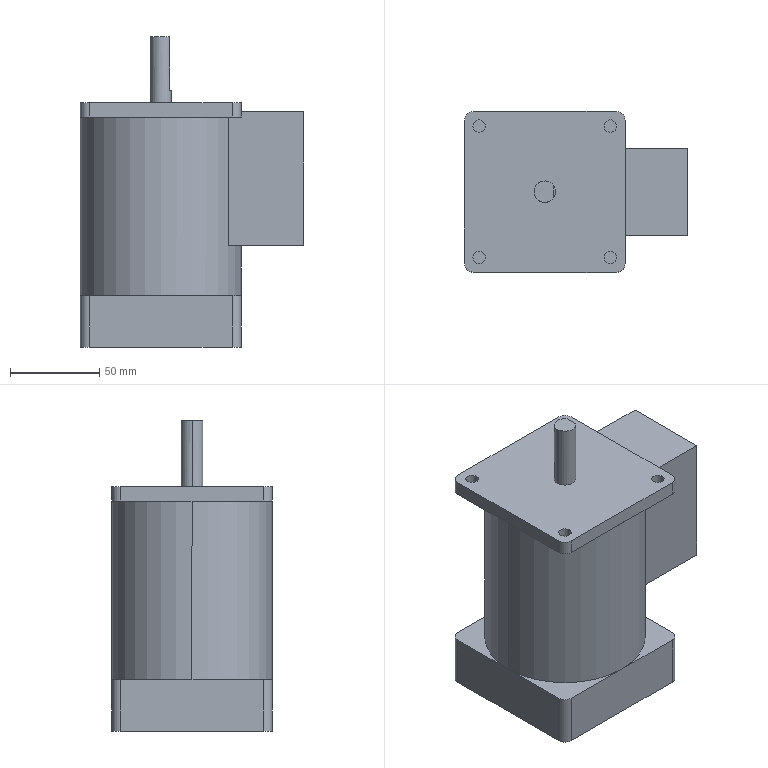Part | SolidWorks | features ICE 6, Fillet 2, CirPattern 1, Extrusion 1 | 1 solid | 46 faces | box 125 x 90 x 174 mm | volume 1074757 mm3 | plane 26 | cylinder 20 | commonest cylinder face diameters 7 x8 10 x8 12 x2 90 x2
STEP:
#1=CARTESIAN_POINT('',(40.27,36.77,0.));
#2=VERTEX_POINT('',#1);
#3=CARTESIAN_POINT('',(33.27,36.77,0.));
#4=VERTEX_POINT('',#3);
#5=CARTESIAN_POINT('',(36.77,36.77,0.));
#6=DIRECTION('',(0.,0.,-1.));
#7=DIRECTION('',(1.,0.,0.));
#8=AXIS2_PLACEMENT_3D('',#5,#6,#7);
#9=CIRCLE('',#8,3.5);
#10=EDGE_CURVE('',#2,#4,#9,.T.);
#11=ORIENTED_EDGE('',*,*,#10,.T.);
#12=CARTESIAN_POINT('',(33.27,36.77,8.));
#13=VERTEX_POINT('',#12);
#14=CARTESIAN_POINT('',(33.27,36.77,-9.899));
#15=DIRECTION('',(0.,0.,1.));
#16=VECTOR('',#15,1000.);
#17=LINE('',#14,#16);
#18=EDGE_CURVE('',#4,#13,#17,.T.);
#19=ORIENTED_EDGE('',*,*,#18,.T.);
#20=CARTESIAN_POINT('',(40.27,36.77,8.));
#21=VERTEX_POINT('',#20);
#22=CARTESIAN_POINT('',(36.77,36.77,8.));
#23=DIRECTION('',(0.,0.,1.));
#24=DIRECTION('',(0.,-1.,0.));
#25=AXIS2_PLACEMENT_3D('',#22,#23,#24);
#26=CIRCLE('',#25,3.5);
#27=EDGE_CURVE('',#13,#21,#26,.T.);
#28=ORIENTED_EDGE('',*,*,#27,.T.);
#29=CARTESIAN_POINT('',(40.27,36.77,-9.899));
#30=DIRECTION('',(0.,0.,1.));
#31=VECTOR('',#30,1000.);
#32=LINE('',#29,#31);
#33=EDGE_CURVE('',#2,#21,#32,.T.);
#34=ORIENTED_EDGE('',*,*,#33,.F.);
#35=EDGE_LOOP('',(#11,#19,#28,#34));
#36=FACE_OUTER_BOUND('',#35,.T.);
#37=CARTESIAN_POINT('',(36.77,36.77,-9.899));
#38=DIRECTION('',(0.,0.,1.));
#39=DIRECTION('',(1.,0.,0.));
#40=AXIS2_PLACEMENT_3D('',#37,#38,#39);
#41=CYLINDRICAL_SURFACE('',#40,3.5);
#42=ADVANCED_FACE('',(#36),#41,.F.);
#43=CARTESIAN_POINT('',(40.27,-36.77,0.));
#44=VERTEX_POINT('',#43);
#45=CARTESIAN_POINT('',(33.27,-36.77,0.));
#46=VERTEX_POINT('',#45);
#47=CARTESIAN_POINT('',(36.77,-36.77,0.));
#48=DIRECTION('',(0.,0.,-1.));
#49=DIRECTION('',(1.,0.,0.));
#50=AXIS2_PLACEMENT_3D('',#47,#48,#49);
#51=CIRCLE('',#50,3.5);
#52=EDGE_CURVE('',#44,#46,#51,.T.);
#53=ORIENTED_EDGE('',*,*,#52,.T.);
#54=CARTESIAN_POINT('',(33.27,-36.77,8.));
#55=VERTEX_POINT('',#54);
#56=CARTESIAN_POINT('',(33.27,-36.77,-9.899));
#57=DIRECTION('',(0.,0.,1.));
#58=VECTOR('',#57,1000.);
#59=LINE('',#56,#58);
#60=EDGE_CURVE('',#46,#55,#59,.T.);
#61=ORIENTED_EDGE('',*,*,#60,.T.);
#62=CARTESIAN_POINT('',(40.27,-36.77,8.));
#63=VERTEX_POINT('',#62);
#64=CARTESIAN_POINT('',(36.77,-36.77,8.));
#65=DIRECTION('',(0.,0.,1.));
#66=DIRECTION('',(-1.,0.,0.));
#67=AXIS2_PLACEMENT_3D('',#64,#65,#66);
#68=CIRCLE('',#67,3.5);
#69=EDGE_CURVE('',#55,#63,#68,.T.);
#70=ORIENTED_EDGE('',*,*,#69,.T.);
#71=CARTESIAN_POINT('',(40.27,-36.77,-9.899));
#72=DIRECTION('',(0.,0.,1.));
#73=VECTOR('',#72,1000.);
#74=LINE('',#71,#73);
#75=EDGE_CURVE('',#44,#63,#74,.T.);
#76=ORIENTED_EDGE('',*,*,#75,.F.);
#77=EDGE_LOOP('',(#53,#61,#70,#76));
#78=FACE_OUTER_BOUND('',#77,.T.);
#79=CARTESIAN_POINT('',(36.77,-36.77,-9.899));
#80=DIRECTION('',(0.,0.,1.));
#81=DIRECTION('',(1.,0.,0.));
#82=AXIS2_PLACEMENT_3D('',#79,#80,#81);
#83=CYLINDRICAL_SURFACE('',#82,3.5);
#84=ADVANCED_FACE('',(#78),#83,.F.);
#85=CARTESIAN_POINT('',(-33.27,-36.77,0.));
#86=VERTEX_POINT('',#85);
#87=CARTESIAN_POINT('',(-40.27,-36.77,0.));
#88=VERTEX_POINT('',#87);
#89=CARTESIAN_POINT('',(-36.77,-36.77,0.));
#90=DIRECTION('',(0.,0.,-1.));
#91=DIRECTION('',(1.,0.,0.));
#92=AXIS2_PLACEMENT_3D('',#89,#90,#91);
#93=CIRCLE('',#92,3.5);
#94=EDGE_CURVE('',#86,#88,#93,.T.);
#95=ORIENTED_EDGE('',*,*,#94,.T.);
#96=CARTESIAN_POINT('',(-40.27,-36.77,8.));
#97=VERTEX_POINT('',#96);
#98=CARTESIAN_POINT('',(-40.27,-36.77,-9.899));
#99=DIRECTION('',(0.,0.,1.));
#100=VECTOR('',#99,1000.);
#101=LINE('',#98,#100);
#102=EDGE_CURVE('',#88,#97,#101,.T.);
#103=ORIENTED_EDGE('',*,*,#102,.T.);
#104=CARTESIAN_POINT('',(-33.27,-36.77,8.));
#105=VERTEX_POINT('',#104);
#106=CARTESIAN_POINT('',(-36.77,-36.77,8.));
#107=DIRECTION('',(0.,0.,1.));
#108=DIRECTION('',(0.,1.,0.));
#109=AXIS2_PLACEMENT_3D('',#106,#107,#108);
#110=CIRCLE('',#109,3.5);
#111=EDGE_CURVE('',#97,#105,#110,.T.);
#112=ORIENTED_EDGE('',*,*,#111,.T.);
#113=CARTESIAN_POINT('',(-33.27,-36.77,-9.899));
#114=DIRECTION('',(0.,0.,1.));
#115=VECTOR('',#114,1000.);
#116=LINE('',#113,#115);
#117=EDGE_CURVE('',#86,#105,#116,.T.);
#118=ORIENTED_EDGE('',*,*,#117,.F.);
#119=EDGE_LOOP('',(#95,#103,#112,#118));
#120=FACE_OUTER_BOUND('',#119,.T.);
#121=CARTESIAN_POINT('',(-36.77,-36.77,-9.899));
#122=DIRECTION('',(0.,0.,1.));
#123=DIRECTION('',(1.,0.,0.));
#124=AXIS2_PLACEMENT_3D('',#121,#122,#123);
#125=CYLINDRICAL_SURFACE('',#124,3.5);
#126=ADVANCED_FACE('',(#120),#125,.F.);
#127=CARTESIAN_POINT('',(-33.27,36.77,0.));
#128=VERTEX_POINT('',#127);
#129=CARTESIAN_POINT('',(-40.27,36.77,0.));
#130=VERTEX_POINT('',#129);
#131=CARTESIAN_POINT('',(-36.77,36.77,0.));
#132=DIRECTION('',(0.,0.,-1.));
#133=DIRECTION('',(1.,0.,0.));
#134=AXIS2_PLACEMENT_3D('',#131,#132,#133);
#135=CIRCLE('',#134,3.5);
#136=EDGE_CURVE('',#128,#130,#135,.T.);
#137=ORIENTED_EDGE('',*,*,#136,.T.);
#138=CARTESIAN_POINT('',(-40.27,36.77,8.));
#139=VERTEX_POINT('',#138);
#140=CARTESIAN_POINT('',(-40.27,36.77,-9.899));
#141=DIRECTION('',(0.,0.,1.));
#142=VECTOR('',#141,1000.);
#143=LINE('',#140,#142);
#144=EDGE_CURVE('',#130,#139,#143,.T.);
#145=ORIENTED_EDGE('',*,*,#144,.T.);
#146=CARTESIAN_POINT('',(-33.27,36.77,8.));
#147=VERTEX_POINT('',#146);
#148=CARTESIAN_POINT('',(-36.77,36.77,8.));
#149=DIRECTION('',(0.,0.,1.));
#150=DIRECTION('',(1.,0.,0.));
#151=AXIS2_PLACEMENT_3D('',#148,#149,#150);
#152=CIRCLE('',#151,3.5);
#153=EDGE_CURVE('',#139,#147,#152,.T.);
#154=ORIENTED_EDGE('',*,*,#153,.T.);
#155=CARTESIAN_POINT('',(-33.27,36.77,-9.899));
#156=DIRECTION('',(0.,0.,1.));
#157=VECTOR('',#156,1000.);
#158=LINE('',#155,#157);
#159=EDGE_CURVE('',#128,#147,#158,.T.);
#160=ORIENTED_EDGE('',*,*,#159,.F.);
#161=EDGE_LOOP('',(#137,#145,#154,#160));
#162=FACE_OUTER_BOUND('',#161,.T.);
#163=CARTESIAN_POINT('',(-36.77,36.77,-9.899));
#164=DIRECTION('',(0.,0.,1.));
#165=DIRECTION('',(1.,0.,0.));
#166=AXIS2_PLACEMENT_3D('',#163,#164,#165);
#167=CYLINDRICAL_SURFACE('',#166,3.5);
#168=ADVANCED_FACE('',(#162),#167,.F.);
#169=CARTESIAN_POINT('',(-45.,0.,-100.));
#170=VERTEX_POINT('',#169);
#171=CARTESIAN_POINT('',(0.,45.,-100.));
#172=VERTEX_POINT('',#171);
#173=CARTESIAN_POINT('',(0.,0.,-100.));
#174=DIRECTION('',(0.,0.,-1.));
#175=DIRECTION('',(-1.,0.,0.));
#176=AXIS2_PLACEMENT_3D('',#173,#174,#175);
#177=CIRCLE('',#176,45.);
#178=EDGE_CURVE('',#170,#172,#177,.T.);
#179=ORIENTED_EDGE('',*,*,#178,.F.);
#180=CARTESIAN_POINT('',(-45.,0.,0.));
#181=VERTEX_POINT('',#180);
#182=CARTESIAN_POINT('',(-45.,0.,-100.));
#183=DIRECTION('',(0.,0.,1.));
#184=VECTOR('',#183,1000.);
#185=LINE('',#182,#184);
#186=EDGE_CURVE('',#170,#181,#185,.T.);
#187=ORIENTED_EDGE('',*,*,#186,.T.);
#188=CARTESIAN_POINT('',(0.,45.,0.));
#189=VERTEX_POINT('',#188);
#190=CARTESIAN_POINT('',(0.,0.,0.));
#191=DIRECTION('',(0.,0.,-1.));
#192=DIRECTION('',(-1.,0.,0.));
#193=AXIS2_PLACEMENT_3D('',#190,#191,#192);
#194=CIRCLE('',#193,45.);
#195=EDGE_CURVE('',#181,#189,#194,.T.);
#196=ORIENTED_EDGE('',*,*,#195,.T.);
#197=CARTESIAN_POINT('',(37.746,24.5,0.));
#198=VERTEX_POINT('',#197);
#199=CARTESIAN_POINT('',(0.,0.,0.));
#200=DIRECTION('',(0.,0.,-1.));
#201=DIRECTION('',(-1.,0.,0.));
#202=AXIS2_PLACEMENT_3D('',#199,#200,#201);
#203=CIRCLE('',#202,45.);
#204=EDGE_CURVE('',#189,#198,#203,.T.);
#205=ORIENTED_EDGE('',*,*,#204,.T.);
#206=CARTESIAN_POINT('',(37.746,24.5,-72.));
#207=VERTEX_POINT('',#206);
#208=CARTESIAN_POINT('',(37.746,24.5,-100.));
#209=DIRECTION('',(0.,0.,1.));
#210=VECTOR('',#209,1000.);
#211=LINE('',#208,#210);
#212=EDGE_CURVE('',#207,#198,#211,.T.);
#213=ORIENTED_EDGE('',*,*,#212,.F.);
#214=CARTESIAN_POINT('',(45.,0.,-72.));
#215=VERTEX_POINT('',#214);
#216=CARTESIAN_POINT('',(0.,0.,-72.));
#217=DIRECTION('',(0.,0.,1.));
#218=DIRECTION('',(1.,0.,0.));
#219=AXIS2_PLACEMENT_3D('',#216,#217,#218);
#220=CIRCLE('',#219,45.);
#221=EDGE_CURVE('',#215,#207,#220,.T.);
#222=ORIENTED_EDGE('',*,*,#221,.F.);
#223=CARTESIAN_POINT('',(45.,0.,-100.));
#224=VERTEX_POINT('',#223);
#225=CARTESIAN_POINT('',(45.,0.,-100.));
#226=DIRECTION('',(0.,0.,1.));
#227=VECTOR('',#226,1000.);
#228=LINE('',#225,#227);
#229=EDGE_CURVE('',#224,#215,#228,.T.);
#230=ORIENTED_EDGE('',*,*,#229,.F.);
#231=CARTESIAN_POINT('',(0.,0.,-100.));
#232=DIRECTION('',(0.,0.,-1.));
#233=DIRECTION('',(-1.,0.,0.));
#234=AXIS2_PLACEMENT_3D('',#231,#232,#233);
#235=CIRCLE('',#234,45.);
#236=EDGE_CURVE('',#172,#224,#235,.T.);
#237=ORIENTED_EDGE('',*,*,#236,.F.);
#238=EDGE_LOOP('',(#179,#187,#196,#205,#213,#222,#230,#237));
#239=FACE_OUTER_BOUND('',#238,.T.);
#240=CARTESIAN_POINT('',(0.,0.,-100.));
#241=DIRECTION('',(0.,0.,1.));
#242=DIRECTION('',(1.,0.,0.));
#243=AXIS2_PLACEMENT_3D('',#240,#241,#242);
#244=CYLINDRICAL_SURFACE('',#243,45.);
#245=ADVANCED_FACE('',(#239),#244,.T.);
#246=CARTESIAN_POINT('',(5.,3.317,15.));
#247=VERTEX_POINT('',#246);
#248=CARTESIAN_POINT('',(6.,0.,15.));
#249=VERTEX_POINT('',#248);
#250=CARTESIAN_POINT('',(0.,0.,15.));
#251=DIRECTION('',(0.,0.,-1.));
#252=DIRECTION('',(0.,1.,0.));
#253=AXIS2_PLACEMENT_3D('',#250,#251,#252);
#254=CIRCLE('',#253,6.);
#255=EDGE_CURVE('',#247,#249,#254,.T.);
#256=ORIENTED_EDGE('',*,*,#255,.T.);
#257=CARTESIAN_POINT('',(6.,0.,8.));
#258=VERTEX_POINT('',#257);
#259=CARTESIAN_POINT('',(6.,0.,45.));
#260=DIRECTION('',(0.,0.,-1.));
#261=VECTOR('',#260,1000.);
#262=LINE('',#259,#261);
#263=EDGE_CURVE('',#249,#258,#262,.T.);
#264=ORIENTED_EDGE('',*,*,#263,.T.);
#265=CARTESIAN_POINT('',(-6.,0.,8.));
#266=VERTEX_POINT('',#265);
#267=CARTESIAN_POINT('',(0.,0.,8.));
#268=DIRECTION('',(0.,0.,1.));
#269=DIRECTION('',(1.,0.,0.));
#270=AXIS2_PLACEMENT_3D('',#267,#268,#269);
#271=CIRCLE('',#270,6.);
#272=EDGE_CURVE('',#258,#266,#271,.T.);
#273=ORIENTED_EDGE('',*,*,#272,.T.);
#274=CARTESIAN_POINT('',(-6.,0.,45.));
#275=VERTEX_POINT('',#274);
#276=CARTESIAN_POINT('',(-6.,0.,45.));
#277=DIRECTION('',(0.,0.,-1.));
#278=VECTOR('',#277,1000.);
#279=LINE('',#276,#278);
#280=EDGE_CURVE('',#275,#266,#279,.T.);
#281=ORIENTED_EDGE('',*,*,#280,.F.);
#282=CARTESIAN_POINT('',(5.,3.317,45.));
#283=VERTEX_POINT('',#282);
#284=CARTESIAN_POINT('',(0.,0.,45.));
#285=DIRECTION('',(0.,0.,1.));
#286=DIRECTION('',(1.,0.,0.));
#287=AXIS2_PLACEMENT_3D('',#284,#285,#286);
#288=CIRCLE('',#287,6.);
#289=EDGE_CURVE('',#283,#275,#288,.T.);
#290=ORIENTED_EDGE('',*,*,#289,.F.);
#291=CARTESIAN_POINT('',(5.,3.317,45.));
#292=DIRECTION('',(0.,0.,1.));
#293=VECTOR('',#292,1000.);
#294=LINE('',#291,#293);
#295=EDGE_CURVE('',#247,#283,#294,.T.);
#296=ORIENTED_EDGE('',*,*,#295,.F.);
#297=EDGE_LOOP('',(#256,#264,#273,#281,#290,#296));
#298=FACE_OUTER_BOUND('',#297,.T.);
#299=CARTESIAN_POINT('',(0.,0.,45.));
#300=DIRECTION('',(0.,0.,-1.));
#301=DIRECTION('',(-1.,0.,0.));
#302=AXIS2_PLACEMENT_3D('',#299,#300,#301);
#303=CYLINDRICAL_SURFACE('',#302,6.);
#304=ADVANCED_FACE('',(#298),#303,.T.);
#305=ORIENTED_EDGE('',*,*,#263,.F.);
#306=CARTESIAN_POINT('',(5.,-3.317,15.));
#307=VERTEX_POINT('',#306);
#308=CARTESIAN_POINT('',(0.,0.,15.));
#309=DIRECTION('',(0.,0.,-1.));
#310=DIRECTION('',(0.,1.,0.));
#311=AXIS2_PLACEMENT_3D('',#308,#309,#310);
#312=CIRCLE('',#311,6.);
#313=EDGE_CURVE('',#249,#307,#312,.T.);
#314=ORIENTED_EDGE('',*,*,#313,.T.);
#315=CARTESIAN_POINT('',(5.,-3.317,45.));
#316=VERTEX_POINT('',#315);
#317=CARTESIAN_POINT('',(5.,-3.317,45.));
#318=DIRECTION('',(0.,0.,-1.));
#319=VECTOR('',#318,1000.);
#320=LINE('',#317,#319);
#321=EDGE_CURVE('',#316,#307,#320,.T.);
#322=ORIENTED_EDGE('',*,*,#321,.F.);
#323=CARTESIAN_POINT('',(0.,0.,45.));
#324=DIRECTION('',(0.,0.,1.));
#325=DIRECTION('',(1.,0.,0.));
#326=AXIS2_PLACEMENT_3D('',#323,#324,#325);
#327=CIRCLE('',#326,6.);
#328=EDGE_CURVE('',#275,#316,#327,.T.);
#329=ORIENTED_EDGE('',*,*,#328,.F.);
#330=ORIENTED_EDGE('',*,*,#280,.T.);
#331=CARTESIAN_POINT('',(0.,0.,8.));
#332=DIRECTION('',(0.,0.,1.));
#333=DIRECTION('',(1.,0.,0.));
#334=AXIS2_PLACEMENT_3D('',#331,#332,#333);
#335=CIRCLE('',#334,6.);
#336=EDGE_CURVE('',#266,#258,#335,.T.);
#337=ORIENTED_EDGE('',*,*,#336,.T.);
#338=EDGE_LOOP('',(#305,#314,#322,#329,#330,#337));
#339=FACE_OUTER_BOUND('',#338,.T.);
#340=CARTESIAN_POINT('',(0.,0.,45.));
#341=DIRECTION('',(0.,0.,-1.));
#342=DIRECTION('',(-1.,0.,0.));
#343=AXIS2_PLACEMENT_3D('',#340,#341,#342);
#344=CYLINDRICAL_SURFACE('',#343,6.);
#345=ADVANCED_FACE('',(#339),#344,.T.);
#346=ORIENTED_EDGE('',*,*,#289,.T.);
#347=ORIENTED_EDGE('',*,*,#328,.T.);
#348=CARTESIAN_POINT('',(5.,0.,45.));
#349=DIRECTION('',(0.,1.,0.));
#350=VECTOR('',#349,1000.);
#351=LINE('',#348,#350);
#352=EDGE_CURVE('',#316,#283,#351,.T.);
#353=ORIENTED_EDGE('',*,*,#352,.T.);
#354=EDGE_LOOP('',(#346,#347,#353));
#355=FACE_OUTER_BOUND('',#354,.T.);
#356=CARTESIAN_POINT('',(0.,0.,45.));
#357=DIRECTION('',(0.,0.,1.));
#358=DIRECTION('',(1.,0.,0.));
#359=AXIS2_PLACEMENT_3D('',#356,#357,#358);
#360=PLANE('',#359);
#361=ADVANCED_FACE('',(#355),#360,.T.);
#362=ORIENTED_EDGE('',*,*,#10,.F.);
#363=CARTESIAN_POINT('',(36.77,36.77,0.));
#364=DIRECTION('',(0.,0.,-1.));
#365=DIRECTION('',(1.,0.,0.));
#366=AXIS2_PLACEMENT_3D('',#363,#364,#365);
#367=CIRCLE('',#366,3.5);
#368=EDGE_CURVE('',#4,#2,#367,.T.);
#369=ORIENTED_EDGE('',*,*,#368,.F.);
#370=EDGE_LOOP('',(#362,#369));
#371=FACE_BOUND('',#370,.T.);
#372=CARTESIAN_POINT('',(40.,45.,0.));
#373=VERTEX_POINT('',#372);
#374=CARTESIAN_POINT('',(-45.,45.,0.));
#375=DIRECTION('',(-1.,0.,0.));
#376=VECTOR('',#375,1000.);
#377=LINE('',#374,#376);
#378=EDGE_CURVE('',#373,#189,#377,.T.);
#379=ORIENTED_EDGE('',*,*,#378,.F.);
#380=CARTESIAN_POINT('',(45.,40.,0.));
#381=VERTEX_POINT('',#380);
#382=CARTESIAN_POINT('',(40.,40.,0.));
#383=DIRECTION('',(0.,0.,-1.));
#384=DIRECTION('',(1.,0.,0.));
#385=AXIS2_PLACEMENT_3D('',#382,#383,#384);
#386=CIRCLE('',#385,5.);
#387=EDGE_CURVE('',#373,#381,#386,.T.);
#388=ORIENTED_EDGE('',*,*,#387,.T.);
#389=CARTESIAN_POINT('',(45.,24.5,0.));
#390=VERTEX_POINT('',#389);
#391=CARTESIAN_POINT('',(45.,45.,0.));
#392=DIRECTION('',(0.,1.,0.));
#393=VECTOR('',#392,1000.);
#394=LINE('',#391,#393);
#395=EDGE_CURVE('',#390,#381,#394,.T.);
#396=ORIENTED_EDGE('',*,*,#395,.F.);
#397=CARTESIAN_POINT('',(-45.,24.5,0.));
#398=DIRECTION('',(1.,0.,0.));
#399=VECTOR('',#398,1000.);
#400=LINE('',#397,#399);
#401=EDGE_CURVE('',#198,#390,#400,.T.);
#402=ORIENTED_EDGE('',*,*,#401,.F.);
#403=ORIENTED_EDGE('',*,*,#204,.F.);
#404=EDGE_LOOP('',(#379,#388,#396,#402,#403));
#405=FACE_OUTER_BOUND('',#404,.T.);
#406=CARTESIAN_POINT('',(-45.,-45.,0.));
#407=DIRECTION('',(0.,0.,1.));
#408=DIRECTION('',(1.,0.,0.));
#409=AXIS2_PLACEMENT_3D('',#406,#407,#408);
#410=PLANE('',#409);
#411=ADVANCED_FACE('',(#371,#405),#410,.F.);
#412=ORIENTED_EDGE('',*,*,#52,.F.);
#413=CARTESIAN_POINT('',(36.77,-36.77,0.));
#414=DIRECTION('',(0.,0.,-1.));
#415=DIRECTION('',(1.,0.,0.));
#416=AXIS2_PLACEMENT_3D('',#413,#414,#415);
#417=CIRCLE('',#416,3.5);
#418=EDGE_CURVE('',#46,#44,#417,.T.);
#419=ORIENTED_EDGE('',*,*,#418,.F.);
#420=EDGE_LOOP('',(#412,#419));
#421=FACE_BOUND('',#420,.T.);
#422=CARTESIAN_POINT('',(45.,-40.,0.));
#423=VERTEX_POINT('',#422);
#424=CARTESIAN_POINT('',(45.,-24.5,0.));
#425=VERTEX_POINT('',#424);
#426=CARTESIAN_POINT('',(45.,45.,0.));
#427=DIRECTION('',(0.,1.,0.));
#428=VECTOR('',#427,1000.);
#429=LINE('',#426,#428);
#430=EDGE_CURVE('',#423,#425,#429,.T.);
#431=ORIENTED_EDGE('',*,*,#430,.F.);
#432=CARTESIAN_POINT('',(40.,-45.,0.));
#433=VERTEX_POINT('',#432);
#434=CARTESIAN_POINT('',(40.,-40.,0.));
#435=DIRECTION('',(0.,0.,-1.));
#436=DIRECTION('',(1.,0.,0.));
#437=AXIS2_PLACEMENT_3D('',#434,#435,#436);
#438=CIRCLE('',#437,5.);
#439=EDGE_CURVE('',#423,#433,#438,.T.);
#440=ORIENTED_EDGE('',*,*,#439,.T.);
#441=CARTESIAN_POINT('',(0.,-45.,0.));
#442=VERTEX_POINT('',#441);
#443=CARTESIAN_POINT('',(-45.,-45.,0.));
#444=DIRECTION('',(1.,0.,0.));
#445=VECTOR('',#444,1000.);
#446=LINE('',#443,#445);
#447=EDGE_CURVE('',#442,#433,#446,.T.);
#448=ORIENTED_EDGE('',*,*,#447,.F.);
#449=CARTESIAN_POINT('',(37.746,-24.5,0.));
#450=VERTEX_POINT('',#449);
#451=CARTESIAN_POINT('',(0.,0.,0.));
#452=DIRECTION('',(0.,0.,-1.));
#453=DIRECTION('',(-1.,0.,0.));
#454=AXIS2_PLACEMENT_3D('',#451,#452,#453);
#455=CIRCLE('',#454,45.);
#456=EDGE_CURVE('',#450,#442,#455,.T.);
#457=ORIENTED_EDGE('',*,*,#456,.F.);
#458=CARTESIAN_POINT('',(-45.,-24.5,0.));
#459=DIRECTION('',(-1.,0.,0.));
#460=VECTOR('',#459,1000.);
#461=LINE('',#458,#460);
#462=EDGE_CURVE('',#425,#450,#461,.T.);
#463=ORIENTED_EDGE('',*,*,#462,.F.);
#464=EDGE_LOOP('',(#431,#440,#448,#457,#463));
#465=FACE_OUTER_BOUND('',#464,.T.);
#466=CARTESIAN_POINT('',(-45.,-45.,0.));
#467=DIRECTION('',(0.,0.,1.));
#468=DIRECTION('',(1.,0.,0.));
#469=AXIS2_PLACEMENT_3D('',#466,#467,#468);
#470=PLANE('',#469);
#471=ADVANCED_FACE('',(#421,#465),#470,.F.);
#472=CARTESIAN_POINT('',(45.,-40.,8.));
#473=VERTEX_POINT('',#472);
#474=CARTESIAN_POINT('',(45.,40.,8.));
#475=VERTEX_POINT('',#474);
#476=CARTESIAN_POINT('',(45.,45.,8.));
#477=DIRECTION('',(0.,1.,0.));
#478=VECTOR('',#477,1000.);
#479=LINE('',#476,#478);
#480=EDGE_CURVE('',#473,#475,#479,.T.);
#481=ORIENTED_EDGE('',*,*,#480,.F.);
#482=CARTESIAN_POINT('',(45.,-40.,8.));
#483=DIRECTION('',(0.,0.,-1.));
#484=VECTOR('',#483,1000.);
#485=LINE('',#482,#484);
#486=EDGE_CURVE('',#473,#423,#485,.T.);
#487=ORIENTED_EDGE('',*,*,#486,.T.);
#488=ORIENTED_EDGE('',*,*,#430,.T.);
#489=CARTESIAN_POINT('',(45.,-24.5,3.));
#490=VERTEX_POINT('',#489);
#491=CARTESIAN_POINT('',(45.,-24.5,8.));
#492=DIRECTION('',(0.,0.,-1.));
#493=VECTOR('',#492,1000.);
#494=LINE('',#491,#493);
#495=EDGE_CURVE('',#490,#425,#494,.T.);
#496=ORIENTED_EDGE('',*,*,#495,.F.);
#497=CARTESIAN_POINT('',(45.,24.5,3.));
#498=VERTEX_POINT('',#497);
#499=CARTESIAN_POINT('',(45.,45.,3.));
#500=DIRECTION('',(0.,-1.,0.));
#501=VECTOR('',#500,1000.);
#502=LINE('',#499,#501);
#503=EDGE_CURVE('',#498,#490,#502,.T.);
#504=ORIENTED_EDGE('',*,*,#503,.F.);
#505=CARTESIAN_POINT('',(45.,24.5,8.));
#506=DIRECTION('',(0.,0.,1.));
#507=VECTOR('',#506,1000.);
#508=LINE('',#505,#507);
#509=EDGE_CURVE('',#390,#498,#508,.T.);
#510=ORIENTED_EDGE('',*,*,#509,.F.);
#511=ORIENTED_EDGE('',*,*,#395,.T.);
#512=CARTESIAN_POINT('',(45.,40.,8.));
#513=DIRECTION('',(0.,0.,1.));
#514=VECTOR('',#513,1000.);
#515=LINE('',#512,#514);
#516=EDGE_CURVE('',#381,#475,#515,.T.);
#517=ORIENTED_EDGE('',*,*,#516,.T.);
#518=EDGE_LOOP('',(#481,#487,#488,#496,#504,#510,#511,#517));
#519=FACE_OUTER_BOUND('',#518,.T.);
#520=CARTESIAN_POINT('',(45.,45.,8.));
#521=DIRECTION('',(-1.,0.,0.));
#522=DIRECTION('',(0.,0.,1.));
#523=AXIS2_PLACEMENT_3D('',#520,#521,#522);
#524=PLANE('',#523);
#525=ADVANCED_FACE('',(#519),#524,.F.);
#526=ORIENTED_EDGE('',*,*,#186,.F.);
#527=CARTESIAN_POINT('',(0.,-45.,-100.));
#528=VERTEX_POINT('',#527);
#529=CARTESIAN_POINT('',(0.,0.,-100.));
#530=DIRECTION('',(0.,0.,-1.));
#531=DIRECTION('',(-1.,0.,0.));
#532=AXIS2_PLACEMENT_3D('',#529,#530,#531);
#533=CIRCLE('',#532,45.);
#534=EDGE_CURVE('',#528,#170,#533,.T.);
#535=ORIENTED_EDGE('',*,*,#534,.F.);
#536=CARTESIAN_POINT('',(0.,0.,-100.));
#537=DIRECTION('',(0.,0.,-1.));
#538=DIRECTION('',(-1.,0.,0.));
#539=AXIS2_PLACEMENT_3D('',#536,#537,#538);
#540=CIRCLE('',#539,45.);
#541=EDGE_CURVE('',#224,#528,#540,.T.);
#542=ORIENTED_EDGE('',*,*,#541,.F.);
#543=ORIENTED_EDGE('',*,*,#229,.T.);
#544=CARTESIAN_POINT('',(37.746,-24.5,-72.));
#545=VERTEX_POINT('',#544);
#546=CARTESIAN_POINT('',(0.,0.,-72.));
#547=DIRECTION('',(0.,0.,1.));
#548=DIRECTION('',(1.,0.,0.));
#549=AXIS2_PLACEMENT_3D('',#546,#547,#548);
#550=CIRCLE('',#549,45.);
#551=EDGE_CURVE('',#545,#215,#550,.T.);
#552=ORIENTED_EDGE('',*,*,#551,.F.);
#553=CARTESIAN_POINT('',(37.746,-24.5,-100.));
#554=DIRECTION('',(0.,0.,-1.));
#555=VECTOR('',#554,1000.);
#556=LINE('',#553,#555);
#557=EDGE_CURVE('',#450,#545,#556,.T.);
#558=ORIENTED_EDGE('',*,*,#557,.F.);
#559=ORIENTED_EDGE('',*,*,#456,.T.);
#560=CARTESIAN_POINT('',(0.,0.,0.));
#561=DIRECTION('',(0.,0.,-1.));
#562=DIRECTION('',(-1.,0.,0.));
#563=AXIS2_PLACEMENT_3D('',#560,#561,#562);
#564=CIRCLE('',#563,45.);
#565=EDGE_CURVE('',#442,#181,#564,.T.);
#566=ORIENTED_EDGE('',*,*,#565,.T.);
#567=EDGE_LOOP('',(#526,#535,#542,#543,#552,#558,#559,#566));
#568=FACE_OUTER_BOUND('',#567,.T.);
#569=CARTESIAN_POINT('',(0.,0.,-100.));
#570=DIRECTION('',(0.,0.,1.));
#571=DIRECTION('',(1.,0.,0.));
#572=AXIS2_PLACEMENT_3D('',#569,#570,#571);
#573=CYLINDRICAL_SURFACE('',#572,45.);
#574=ADVANCED_FACE('',(#568),#573,.T.);
#575=CARTESIAN_POINT('',(36.77,36.77,8.));
#576=DIRECTION('',(0.,0.,1.));
#577=DIRECTION('',(0.,-1.,0.));
#578=AXIS2_PLACEMENT_3D('',#575,#576,#577);
#579=CIRCLE('',#578,3.5);
#580=EDGE_CURVE('',#21,#13,#579,.T.);
#581=ORIENTED_EDGE('',*,*,#580,.F.);
#582=ORIENTED_EDGE('',*,*,#27,.F.);
#583=EDGE_LOOP('',(#581,#582));
#584=FACE_BOUND('',#583,.T.);
#585=CARTESIAN_POINT('',(36.77,-36.77,8.));
#586=DIRECTION('',(0.,0.,1.));
#587=DIRECTION('',(-1.,0.,0.));
#588=AXIS2_PLACEMENT_3D('',#585,#586,#587);
#589=CIRCLE('',#588,3.5);
#590=EDGE_CURVE('',#63,#55,#589,.T.);
#591=ORIENTED_EDGE('',*,*,#590,.F.);
#592=ORIENTED_EDGE('',*,*,#69,.F.);
#593=EDGE_LOOP('',(#591,#592));
#594=FACE_BOUND('',#593,.T.);
#595=CARTESIAN_POINT('',(-36.77,-36.77,8.));
#596=DIRECTION('',(0.,0.,1.));
#597=DIRECTION('',(0.,1.,0.));
#598=AXIS2_PLACEMENT_3D('',#595,#596,#597);
#599=CIRCLE('',#598,3.5);
#600=EDGE_CURVE('',#105,#97,#599,.T.);
#601=ORIENTED_EDGE('',*,*,#600,.F.);
#602=ORIENTED_EDGE('',*,*,#111,.F.);
#603=EDGE_LOOP('',(#601,#602));
#604=FACE_BOUND('',#603,.T.);
#605=CARTESIAN_POINT('',(-36.77,36.77,8.));
#606=DIRECTION('',(0.,0.,1.));
#607=DIRECTION('',(1.,0.,0.));
#608=AXIS2_PLACEMENT_3D('',#605,#606,#607);
#609=CIRCLE('',#608,3.5);
#610=EDGE_CURVE('',#147,#139,#609,.T.);
#611=ORIENTED_EDGE('',*,*,#610,.F.);
#612=ORIENTED_EDGE('',*,*,#153,.F.);
#613=EDGE_LOOP('',(#611,#612));
#614=FACE_BOUND('',#613,.T.);
#615=CARTESIAN_POINT('',(-40.,-45.,8.));
#616=VERTEX_POINT('',#615);
#617=CARTESIAN_POINT('',(40.,-45.,8.));
#618=VERTEX_POINT('',#617);
#619=CARTESIAN_POINT('',(-45.,-45.,8.));
#620=DIRECTION('',(1.,0.,0.));
#621=VECTOR('',#620,1000.);
#622=LINE('',#619,#621);
#623=EDGE_CURVE('',#616,#618,#622,.T.);
#624=ORIENTED_EDGE('',*,*,#623,.T.);
#625=CARTESIAN_POINT('',(40.,-40.,8.));
#626=DIRECTION('',(0.,0.,1.));
#627=DIRECTION('',(1.,0.,0.));
#628=AXIS2_PLACEMENT_3D('',#625,#626,#627);
#629=CIRCLE('',#628,5.);
#630=EDGE_CURVE('',#618,#473,#629,.T.);
#631=ORIENTED_EDGE('',*,*,#630,.T.);
#632=ORIENTED_EDGE('',*,*,#480,.T.);
#633=CARTESIAN_POINT('',(40.,45.,8.));
#634=VERTEX_POINT('',#633);
#635=CARTESIAN_POINT('',(40.,40.,8.));
#636=DIRECTION('',(0.,0.,1.));
#637=DIRECTION('',(1.,0.,0.));
#638=AXIS2_PLACEMENT_3D('',#635,#636,#637);
#639=CIRCLE('',#638,5.);
#640=EDGE_CURVE('',#475,#634,#639,.T.);
#641=ORIENTED_EDGE('',*,*,#640,.T.);
#642=CARTESIAN_POINT('',(-40.,45.,8.));
#643=VERTEX_POINT('',#642);
#644=CARTESIAN_POINT('',(-45.,45.,8.));
#645=DIRECTION('',(-1.,0.,0.));
#646=VECTOR('',#645,1000.);
#647=LINE('',#644,#646);
#648=EDGE_CURVE('',#634,#643,#647,.T.);
#649=ORIENTED_EDGE('',*,*,#648,.T.);
#650=CARTESIAN_POINT('',(-45.,40.,8.));
#651=VERTEX_POINT('',#650);
#652=CARTESIAN_POINT('',(-40.,40.,8.));
#653=DIRECTION('',(0.,0.,1.));
#654=DIRECTION('',(1.,0.,0.));
#655=AXIS2_PLACEMENT_3D('',#652,#653,#654);
#656=CIRCLE('',#655,5.);
#657=EDGE_CURVE('',#643,#651,#656,.T.);
#658=ORIENTED_EDGE('',*,*,#657,.T.);
#659=CARTESIAN_POINT('',(-45.,-40.,8.));
#660=VERTEX_POINT('',#659);
#661=CARTESIAN_POINT('',(-45.,45.,8.));
#662=DIRECTION('',(0.,-1.,0.));
#663=VECTOR('',#662,1000.);
#664=LINE('',#661,#663);
#665=EDGE_CURVE('',#651,#660,#664,.T.);
#666=ORIENTED_EDGE('',*,*,#665,.T.);
#667=CARTESIAN_POINT('',(-40.,-40.,8.));
#668=DIRECTION('',(0.,0.,1.));
#669=DIRECTION('',(1.,0.,0.));
#670=AXIS2_PLACEMENT_3D('',#667,#668,#669);
#671=CIRCLE('',#670,5.);
#672=EDGE_CURVE('',#660,#616,#671,.T.);
#673=ORIENTED_EDGE('',*,*,#672,.T.);
#674=EDGE_LOOP('',(#624,#631,#632,#641,#649,#658,#666,#673));
#675=FACE_OUTER_BOUND('',#674,.T.);
#676=ORIENTED_EDGE('',*,*,#336,.F.);
#677=ORIENTED_EDGE('',*,*,#272,.F.);
#678=EDGE_LOOP('',(#676,#677));
#679=FACE_BOUND('',#678,.T.);
#680=CARTESIAN_POINT('',(-45.,-45.,8.));
#681=DIRECTION('',(0.,0.,1.));
#682=DIRECTION('',(1.,0.,0.));
#683=AXIS2_PLACEMENT_3D('',#680,#681,#682);
#684=PLANE('',#683);
#685=ADVANCED_FACE('',(#584,#594,#604,#614,#675,#679),#684,.T.);
#686=ORIENTED_EDGE('',*,*,#136,.F.);
#687=CARTESIAN_POINT('',(-36.77,36.77,0.));
#688=DIRECTION('',(0.,0.,-1.));
#689=DIRECTION('',(1.,0.,0.));
#690=AXIS2_PLACEMENT_3D('',#687,#688,#689);
#691=CIRCLE('',#690,3.5);
#692=EDGE_CURVE('',#130,#128,#691,.T.);
#693=ORIENTED_EDGE('',*,*,#692,.F.);
#694=EDGE_LOOP('',(#686,#693));
#695=FACE_BOUND('',#694,.T.);
#696=CARTESIAN_POINT('',(-45.,40.,0.));
#697=VERTEX_POINT('',#696);
#698=CARTESIAN_POINT('',(-45.,45.,0.));
#699=DIRECTION('',(0.,-1.,0.));
#700=VECTOR('',#699,1000.);
#701=LINE('',#698,#700);
#702=EDGE_CURVE('',#697,#181,#701,.T.);
#703=ORIENTED_EDGE('',*,*,#702,.F.);
#704=CARTESIAN_POINT('',(-40.,45.,0.));
#705=VERTEX_POINT('',#704);
#706=CARTESIAN_POINT('',(-40.,40.,0.));
#707=DIRECTION('',(0.,0.,-1.));
#708=DIRECTION('',(1.,0.,0.));
#709=AXIS2_PLACEMENT_3D('',#706,#707,#708);
#710=CIRCLE('',#709,5.);
#711=EDGE_CURVE('',#697,#705,#710,.T.);
#712=ORIENTED_EDGE('',*,*,#711,.T.);
#713=CARTESIAN_POINT('',(-45.,45.,0.));
#714=DIRECTION('',(-1.,0.,0.));
#715=VECTOR('',#714,1000.);
#716=LINE('',#713,#715);
#717=EDGE_CURVE('',#189,#705,#716,.T.);
#718=ORIENTED_EDGE('',*,*,#717,.F.);
#719=ORIENTED_EDGE('',*,*,#195,.F.);
#720=EDGE_LOOP('',(#703,#712,#718,#719));
#721=FACE_OUTER_BOUND('',#720,.T.);
#722=CARTESIAN_POINT('',(-45.,-45.,0.));
#723=DIRECTION('',(0.,0.,1.));
#724=DIRECTION('',(1.,0.,0.));
#725=AXIS2_PLACEMENT_3D('',#722,#723,#724);
#726=PLANE('',#725);
#727=ADVANCED_FACE('',(#695,#721),#726,.F.);
#728=ORIENTED_EDGE('',*,*,#94,.F.);
#729=CARTESIAN_POINT('',(-36.77,-36.77,0.));
#730=DIRECTION('',(0.,0.,-1.));
#731=DIRECTION('',(1.,0.,0.));
#732=AXIS2_PLACEMENT_3D('',#729,#730,#731);
#733=CIRCLE('',#732,3.5);
#734=EDGE_CURVE('',#88,#86,#733,.T.);
#735=ORIENTED_EDGE('',*,*,#734,.F.);
#736=EDGE_LOOP('',(#728,#735));
#737=FACE_BOUND('',#736,.T.);
#738=CARTESIAN_POINT('',(-40.,-45.,0.));
#739=VERTEX_POINT('',#738);
#740=CARTESIAN_POINT('',(-45.,-45.,0.));
#741=DIRECTION('',(1.,0.,0.));
#742=VECTOR('',#741,1000.);
#743=LINE('',#740,#742);
#744=EDGE_CURVE('',#739,#442,#743,.T.);
#745=ORIENTED_EDGE('',*,*,#744,.F.);
#746=CARTESIAN_POINT('',(-45.,-40.,0.));
#747=VERTEX_POINT('',#746);
#748=CARTESIAN_POINT('',(-40.,-40.,0.));
#749=DIRECTION('',(0.,0.,-1.));
#750=DIRECTION('',(1.,0.,0.));
#751=AXIS2_PLACEMENT_3D('',#748,#749,#750);
#752=CIRCLE('',#751,5.);
#753=EDGE_CURVE('',#739,#747,#752,.T.);
#754=ORIENTED_EDGE('',*,*,#753,.T.);
#755=CARTESIAN_POINT('',(-45.,45.,0.));
#756=DIRECTION('',(0.,-1.,0.));
#757=VECTOR('',#756,1000.);
#758=LINE('',#755,#757);
#759=EDGE_CURVE('',#181,#747,#758,.T.);
#760=ORIENTED_EDGE('',*,*,#759,.F.);
#761=ORIENTED_EDGE('',*,*,#565,.F.);
#762=EDGE_LOOP('',(#745,#754,#760,#761));
#763=FACE_OUTER_BOUND('',#762,.T.);
#764=CARTESIAN_POINT('',(-45.,-45.,0.));
#765=DIRECTION('',(0.,0.,1.));
#766=DIRECTION('',(1.,0.,0.));
#767=AXIS2_PLACEMENT_3D('',#764,#765,#766);
#768=PLANE('',#767);
#769=ADVANCED_FACE('',(#737,#763),#768,.F.);
#770=ORIENTED_EDGE('',*,*,#759,.T.);
#771=CARTESIAN_POINT('',(-45.,-40.,8.));
#772=DIRECTION('',(0.,0.,1.));
#773=VECTOR('',#772,1000.);
#774=LINE('',#771,#773);
#775=EDGE_CURVE('',#747,#660,#774,.T.);
#776=ORIENTED_EDGE('',*,*,#775,.T.);
#777=ORIENTED_EDGE('',*,*,#665,.F.);
#778=CARTESIAN_POINT('',(-45.,40.,8.));
#779=DIRECTION('',(0.,0.,-1.));
#780=VECTOR('',#779,1000.);
#781=LINE('',#778,#780);
#782=EDGE_CURVE('',#651,#697,#781,.T.);
#783=ORIENTED_EDGE('',*,*,#782,.T.);
#784=ORIENTED_EDGE('',*,*,#702,.T.);
#785=EDGE_LOOP('',(#770,#776,#777,#783,#784));
#786=FACE_OUTER_BOUND('',#785,.T.);
#787=CARTESIAN_POINT('',(-45.,45.,8.));
#788=DIRECTION('',(1.,0.,0.));
#789=DIRECTION('',(0.,0.,-1.));
#790=AXIS2_PLACEMENT_3D('',#787,#788,#789);
#791=PLANE('',#790);
#792=ADVANCED_FACE('',(#786),#791,.F.);
#793=ORIENTED_EDGE('',*,*,#447,.T.);
#794=CARTESIAN_POINT('',(40.,-45.,8.));
#795=DIRECTION('',(0.,0.,1.));
#796=VECTOR('',#795,1000.);
#797=LINE('',#794,#796);
#798=EDGE_CURVE('',#433,#618,#797,.T.);
#799=ORIENTED_EDGE('',*,*,#798,.T.);
#800=ORIENTED_EDGE('',*,*,#623,.F.);
#801=CARTESIAN_POINT('',(-40.,-45.,8.));
#802=DIRECTION('',(0.,0.,-1.));
#803=VECTOR('',#802,1000.);
#804=LINE('',#801,#803);
#805=EDGE_CURVE('',#616,#739,#804,.T.);
#806=ORIENTED_EDGE('',*,*,#805,.T.);
#807=ORIENTED_EDGE('',*,*,#744,.T.);
#808=EDGE_LOOP('',(#793,#799,#800,#806,#807));
#809=FACE_OUTER_BOUND('',#808,.T.);
#810=CARTESIAN_POINT('',(-45.,-45.,8.));
#811=DIRECTION('',(0.,1.,0.));
#812=DIRECTION('',(0.,0.,1.));
#813=AXIS2_PLACEMENT_3D('',#810,#811,#812);
#814=PLANE('',#813);
#815=ADVANCED_FACE('',(#809),#814,.F.);
#816=ORIENTED_EDGE('',*,*,#648,.F.);
#817=CARTESIAN_POINT('',(40.,45.,8.));
#818=DIRECTION('',(0.,0.,-1.));
#819=VECTOR('',#818,1000.);
#820=LINE('',#817,#819);
#821=EDGE_CURVE('',#634,#373,#820,.T.);
#822=ORIENTED_EDGE('',*,*,#821,.T.);
#823=ORIENTED_EDGE('',*,*,#378,.T.);
#824=ORIENTED_EDGE('',*,*,#717,.T.);
#825=CARTESIAN_POINT('',(-40.,45.,8.));
#826=DIRECTION('',(0.,0.,1.));
#827=VECTOR('',#826,1000.);
#828=LINE('',#825,#827);
#829=EDGE_CURVE('',#705,#643,#828,.T.);
#830=ORIENTED_EDGE('',*,*,#829,.T.);
#831=EDGE_LOOP('',(#816,#822,#823,#824,#830));
#832=FACE_OUTER_BOUND('',#831,.T.);
#833=CARTESIAN_POINT('',(-45.,45.,8.));
#834=DIRECTION('',(0.,-1.,0.));
#835=DIRECTION('',(0.,0.,-1.));
#836=AXIS2_PLACEMENT_3D('',#833,#834,#835);
#837=PLANE('',#836);
#838=ADVANCED_FACE('',(#832),#837,.F.);
#839=CARTESIAN_POINT('',(-40.,45.,-100.));
#840=VERTEX_POINT('',#839);
#841=CARTESIAN_POINT('',(45.,45.,-100.));
#842=DIRECTION('',(1.,0.,0.));
#843=VECTOR('',#842,1000.);
#844=LINE('',#841,#843);
#845=EDGE_CURVE('',#840,#172,#844,.T.);
#846=ORIENTED_EDGE('',*,*,#845,.F.);
#847=CARTESIAN_POINT('',(-45.,40.,-100.));
#848=VERTEX_POINT('',#847);
#849=CARTESIAN_POINT('',(-40.,40.,-100.));
#850=DIRECTION('',(0.,0.,1.));
#851=DIRECTION('',(-1.,0.,0.));
#852=AXIS2_PLACEMENT_3D('',#849,#850,#851);
#853=CIRCLE('',#852,5.);
#854=EDGE_CURVE('',#840,#848,#853,.T.);
#855=ORIENTED_EDGE('',*,*,#854,.T.);
#856=CARTESIAN_POINT('',(-45.,45.,-100.));
#857=DIRECTION('',(0.,1.,0.));
#858=VECTOR('',#857,1000.);
#859=LINE('',#856,#858);
#860=EDGE_CURVE('',#170,#848,#859,.T.);
#861=ORIENTED_EDGE('',*,*,#860,.F.);
#862=ORIENTED_EDGE('',*,*,#178,.T.);
#863=EDGE_LOOP('',(#846,#855,#861,#862));
#864=FACE_OUTER_BOUND('',#863,.T.);
#865=CARTESIAN_POINT('',(45.,-45.,-100.));
#866=DIRECTION('',(0.,0.,-1.));
#867=DIRECTION('',(-1.,0.,0.));
#868=AXIS2_PLACEMENT_3D('',#865,#866,#867);
#869=PLANE('',#868);
#870=ADVANCED_FACE('',(#864),#869,.F.);
#871=CARTESIAN_POINT('',(45.,40.,-100.));
#872=VERTEX_POINT('',#871);
#873=CARTESIAN_POINT('',(45.,45.,-100.));
#874=DIRECTION('',(0.,-1.,0.));
#875=VECTOR('',#874,1000.);
#876=LINE('',#873,#875);
#877=EDGE_CURVE('',#872,#224,#876,.T.);
#878=ORIENTED_EDGE('',*,*,#877,.F.);
#879=CARTESIAN_POINT('',(40.,45.,-100.));
#880=VERTEX_POINT('',#879);
#881=CARTESIAN_POINT('',(40.,40.,-100.));
#882=DIRECTION('',(0.,0.,1.));
#883=DIRECTION('',(-1.,0.,0.));
#884=AXIS2_PLACEMENT_3D('',#881,#882,#883);
#885=CIRCLE('',#884,5.);
#886=EDGE_CURVE('',#872,#880,#885,.T.);
#887=ORIENTED_EDGE('',*,*,#886,.T.);
#888=CARTESIAN_POINT('',(45.,45.,-100.));
#889=DIRECTION('',(1.,0.,0.));
#890=VECTOR('',#889,1000.);
#891=LINE('',#888,#890);
#892=EDGE_CURVE('',#172,#880,#891,.T.);
#893=ORIENTED_EDGE('',*,*,#892,.F.);
#894=ORIENTED_EDGE('',*,*,#236,.T.);
#895=EDGE_LOOP('',(#878,#887,#893,#894));
#896=FACE_OUTER_BOUND('',#895,.T.);
#897=CARTESIAN_POINT('',(45.,-45.,-100.));
#898=DIRECTION('',(0.,0.,-1.));
#899=DIRECTION('',(-1.,0.,0.));
#900=AXIS2_PLACEMENT_3D('',#897,#898,#899);
#901=PLANE('',#900);
#902=ADVANCED_FACE('',(#896),#901,.F.);
#903=CARTESIAN_POINT('',(40.,-45.,-100.));
#904=VERTEX_POINT('',#903);
#905=CARTESIAN_POINT('',(45.,-45.,-100.));
#906=DIRECTION('',(-1.,0.,0.));
#907=VECTOR('',#906,1000.);
#908=LINE('',#905,#907);
#909=EDGE_CURVE('',#904,#528,#908,.T.);
#910=ORIENTED_EDGE('',*,*,#909,.F.);
#911=CARTESIAN_POINT('',(45.,-40.,-100.));
#912=VERTEX_POINT('',#911);
#913=CARTESIAN_POINT('',(40.,-40.,-100.));
#914=DIRECTION('',(0.,0.,1.));
#915=DIRECTION('',(-1.,0.,0.));
#916=AXIS2_PLACEMENT_3D('',#913,#914,#915);
#917=CIRCLE('',#916,5.);
#918=EDGE_CURVE('',#904,#912,#917,.T.);
#919=ORIENTED_EDGE('',*,*,#918,.T.);
#920=CARTESIAN_POINT('',(45.,45.,-100.));
#921=DIRECTION('',(0.,-1.,0.));
#922=VECTOR('',#921,1000.);
#923=LINE('',#920,#922);
#924=EDGE_CURVE('',#224,#912,#923,.T.);
#925=ORIENTED_EDGE('',*,*,#924,.F.);
#926=ORIENTED_EDGE('',*,*,#541,.T.);
#927=EDGE_LOOP('',(#910,#919,#925,#926));
#928=FACE_OUTER_BOUND('',#927,.T.);
#929=CARTESIAN_POINT('',(45.,-45.,-100.));
#930=DIRECTION('',(0.,0.,-1.));
#931=DIRECTION('',(-1.,0.,0.));
#932=AXIS2_PLACEMENT_3D('',#929,#930,#931);
#933=PLANE('',#932);
#934=ADVANCED_FACE('',(#928),#933,.F.);
#935=CARTESIAN_POINT('',(-45.,-40.,-100.));
#936=VERTEX_POINT('',#935);
#937=CARTESIAN_POINT('',(-45.,45.,-100.));
#938=DIRECTION('',(0.,1.,0.));
#939=VECTOR('',#938,1000.);
#940=LINE('',#937,#939);
#941=EDGE_CURVE('',#936,#170,#940,.T.);
#942=ORIENTED_EDGE('',*,*,#941,.F.);
#943=CARTESIAN_POINT('',(-40.,-45.,-100.));
#944=VERTEX_POINT('',#943);
#945=CARTESIAN_POINT('',(-40.,-40.,-100.));
#946=DIRECTION('',(0.,0.,1.));
#947=DIRECTION('',(-1.,0.,0.));
#948=AXIS2_PLACEMENT_3D('',#945,#946,#947);
#949=CIRCLE('',#948,5.);
#950=EDGE_CURVE('',#936,#944,#949,.T.);
#951=ORIENTED_EDGE('',*,*,#950,.T.);
#952=CARTESIAN_POINT('',(45.,-45.,-100.));
#953=DIRECTION('',(-1.,0.,0.));
#954=VECTOR('',#953,1000.);
#955=LINE('',#952,#954);
#956=EDGE_CURVE('',#528,#944,#955,.T.);
#957=ORIENTED_EDGE('',*,*,#956,.F.);
#958=ORIENTED_EDGE('',*,*,#534,.T.);
#959=EDGE_LOOP('',(#942,#951,#957,#958));
#960=FACE_OUTER_BOUND('',#959,.T.);
#961=CARTESIAN_POINT('',(45.,-45.,-100.));
#962=DIRECTION('',(0.,0.,-1.));
#963=DIRECTION('',(-1.,0.,0.));
#964=AXIS2_PLACEMENT_3D('',#961,#962,#963);
#965=PLANE('',#964);
#966=ADVANCED_FACE('',(#960),#965,.F.);
#967=ORIENTED_EDGE('',*,*,#924,.T.);
#968=CARTESIAN_POINT('',(45.,-40.,-129.));
#969=VERTEX_POINT('',#968);
#970=CARTESIAN_POINT('',(45.,-40.,-129.));
#971=DIRECTION('',(0.,0.,-1.));
#972=VECTOR('',#971,1000.);
#973=LINE('',#970,#972);
#974=EDGE_CURVE('',#912,#969,#973,.T.);
#975=ORIENTED_EDGE('',*,*,#974,.T.);
#976=CARTESIAN_POINT('',(45.,40.,-129.));
#977=VERTEX_POINT('',#976);
#978=CARTESIAN_POINT('',(45.,45.,-129.));
#979=DIRECTION('',(0.,-1.,0.));
#980=VECTOR('',#979,1000.);
#981=LINE('',#978,#980);
#982=EDGE_CURVE('',#977,#969,#981,.T.);
#983=ORIENTED_EDGE('',*,*,#982,.F.);
#984=CARTESIAN_POINT('',(45.,40.,-129.));
#985=DIRECTION('',(0.,0.,1.));
#986=VECTOR('',#985,1000.);
#987=LINE('',#984,#986);
#988=EDGE_CURVE('',#977,#872,#987,.T.);
#989=ORIENTED_EDGE('',*,*,#988,.T.);
#990=ORIENTED_EDGE('',*,*,#877,.T.);
#991=EDGE_LOOP('',(#967,#975,#983,#989,#990));
#992=FACE_OUTER_BOUND('',#991,.T.);
#993=CARTESIAN_POINT('',(45.,45.,-129.));
#994=DIRECTION('',(-1.,0.,0.));
#995=DIRECTION('',(0.,-1.,0.));
#996=AXIS2_PLACEMENT_3D('',#993,#994,#995);
#997=PLANE('',#996);
#998=ADVANCED_FACE('',(#992),#997,.F.);
#999=CARTESIAN_POINT('',(40.,-45.,-129.));
#1000=VERTEX_POINT('',#999);
#1001=CARTESIAN_POINT('',(-40.,-45.,-129.));
#1002=VERTEX_POINT('',#1001);
#1003=CARTESIAN_POINT('',(45.,-45.,-129.));
#1004=DIRECTION('',(-1.,0.,0.));
#1005=VECTOR('',#1004,1000.);
#1006=LINE('',#1003,#1005);
#1007=EDGE_CURVE('',#1000,#1002,#1006,.T.);
#1008=ORIENTED_EDGE('',*,*,#1007,.F.);
#1009=CARTESIAN_POINT('',(40.,-45.,-129.));
#1010=DIRECTION('',(0.,0.,1.));
#1011=VECTOR('',#1010,1000.);
#1012=LINE('',#1009,#1011);
#1013=EDGE_CURVE('',#1000,#904,#1012,.T.);
#1014=ORIENTED_EDGE('',*,*,#1013,.T.);
#1015=ORIENTED_EDGE('',*,*,#909,.T.);
#1016=ORIENTED_EDGE('',*,*,#956,.T.);
#1017=CARTESIAN_POINT('',(-40.,-45.,-129.));
#1018=DIRECTION('',(0.,0.,-1.));
#1019=VECTOR('',#1018,1000.);
#1020=LINE('',#1017,#1019);
#1021=EDGE_CURVE('',#944,#1002,#1020,.T.);
#1022=ORIENTED_EDGE('',*,*,#1021,.T.);
#1023=EDGE_LOOP('',(#1008,#1014,#1015,#1016,#1022));
#1024=FACE_OUTER_BOUND('',#1023,.T.);
#1025=CARTESIAN_POINT('',(45.,-45.,-129.));
#1026=DIRECTION('',(0.,1.,0.));
#1027=DIRECTION('',(-1.,0.,0.));
#1028=AXIS2_PLACEMENT_3D('',#1025,#1026,#1027);
#1029=PLANE('',#1028);
#1030=ADVANCED_FACE('',(#1024),#1029,.F.);
#1031=CARTESIAN_POINT('',(-45.,-40.,-129.));
#1032=VERTEX_POINT('',#1031);
#1033=CARTESIAN_POINT('',(-45.,40.,-129.));
#1034=VERTEX_POINT('',#1033);
#1035=CARTESIAN_POINT('',(-45.,45.,-129.));
#1036=DIRECTION('',(0.,1.,0.));
#1037=VECTOR('',#1036,1000.);
#1038=LINE('',#1035,#1037);
#1039=EDGE_CURVE('',#1032,#1034,#1038,.T.);
#1040=ORIENTED_EDGE('',*,*,#1039,.F.);
#1041=CARTESIAN_POINT('',(-45.,-40.,-129.));
#1042=DIRECTION('',(0.,0.,1.));
#1043=VECTOR('',#1042,1000.);
#1044=LINE('',#1041,#1043);
#1045=EDGE_CURVE('',#1032,#936,#1044,.T.);
#1046=ORIENTED_EDGE('',*,*,#1045,.T.);
#1047=ORIENTED_EDGE('',*,*,#941,.T.);
#1048=ORIENTED_EDGE('',*,*,#860,.T.);
#1049=CARTESIAN_POINT('',(-45.,40.,-129.));
#1050=DIRECTION('',(0.,0.,-1.));
#1051=VECTOR('',#1050,1000.);
#1052=LINE('',#1049,#1051);
#1053=EDGE_CURVE('',#848,#1034,#1052,.T.);
#1054=ORIENTED_EDGE('',*,*,#1053,.T.);
#1055=EDGE_LOOP('',(#1040,#1046,#1047,#1048,#1054));
#1056=FACE_OUTER_BOUND('',#1055,.T.);
#1057=CARTESIAN_POINT('',(-45.,45.,-129.));
#1058=DIRECTION('',(1.,0.,0.));
#1059=DIRECTION('',(0.,1.,0.));
#1060=AXIS2_PLACEMENT_3D('',#1057,#1058,#1059);
#1061=PLANE('',#1060);
#1062=ADVANCED_FACE('',(#1056),#1061,.F.);
#1063=ORIENTED_EDGE('',*,*,#892,.T.);
#1064=CARTESIAN_POINT('',(40.,45.,-129.));
#1065=VERTEX_POINT('',#1064);
#1066=CARTESIAN_POINT('',(40.,45.,-129.));
#1067=DIRECTION('',(0.,0.,-1.));
#1068=VECTOR('',#1067,1000.);
#1069=LINE('',#1066,#1068);
#1070=EDGE_CURVE('',#880,#1065,#1069,.T.);
#1071=ORIENTED_EDGE('',*,*,#1070,.T.);
#1072=CARTESIAN_POINT('',(-40.,45.,-129.));
#1073=VERTEX_POINT('',#1072);
#1074=CARTESIAN_POINT('',(45.,45.,-129.));
#1075=DIRECTION('',(1.,0.,0.));
#1076=VECTOR('',#1075,1000.);
#1077=LINE('',#1074,#1076);
#1078=EDGE_CURVE('',#1073,#1065,#1077,.T.);
#1079=ORIENTED_EDGE('',*,*,#1078,.F.);
#1080=CARTESIAN_POINT('',(-40.,45.,-129.));
#1081=DIRECTION('',(0.,0.,1.));
#1082=VECTOR('',#1081,1000.);
#1083=LINE('',#1080,#1082);
#1084=EDGE_CURVE('',#1073,#840,#1083,.T.);
#1085=ORIENTED_EDGE('',*,*,#1084,.T.);
#1086=ORIENTED_EDGE('',*,*,#845,.T.);
#1087=EDGE_LOOP('',(#1063,#1071,#1079,#1085,#1086));
#1088=FACE_OUTER_BOUND('',#1087,.T.);
#1089=CARTESIAN_POINT('',(45.,45.,-129.));
#1090=DIRECTION('',(0.,-1.,0.));
#1091=DIRECTION('',(1.,0.,0.));
#1092=AXIS2_PLACEMENT_3D('',#1089,#1090,#1091);
#1093=PLANE('',#1092);
#1094=ADVANCED_FACE('',(#1088),#1093,.F.);
#1095=ORIENTED_EDGE('',*,*,#982,.T.);
#1096=CARTESIAN_POINT('',(40.,-40.,-129.));
#1097=DIRECTION('',(0.,0.,-1.));
#1098=DIRECTION('',(-1.,0.,0.));
#1099=AXIS2_PLACEMENT_3D('',#1096,#1097,#1098);
#1100=CIRCLE('',#1099,5.);
#1101=EDGE_CURVE('',#969,#1000,#1100,.T.);
#1102=ORIENTED_EDGE('',*,*,#1101,.T.);
#1103=ORIENTED_EDGE('',*,*,#1007,.T.);
#1104=CARTESIAN_POINT('',(-40.,-40.,-129.));
#1105=DIRECTION('',(0.,0.,-1.));
#1106=DIRECTION('',(-1.,0.,0.));
#1107=AXIS2_PLACEMENT_3D('',#1104,#1105,#1106);
#1108=CIRCLE('',#1107,5.);
#1109=EDGE_CURVE('',#1002,#1032,#1108,.T.);
#1110=ORIENTED_EDGE('',*,*,#1109,.T.);
#1111=ORIENTED_EDGE('',*,*,#1039,.T.);
#1112=CARTESIAN_POINT('',(-40.,40.,-129.));
#1113=DIRECTION('',(0.,0.,-1.));
#1114=DIRECTION('',(-1.,0.,0.));
#1115=AXIS2_PLACEMENT_3D('',#1112,#1113,#1114);
#1116=CIRCLE('',#1115,5.);
#1117=EDGE_CURVE('',#1034,#1073,#1116,.T.);
#1118=ORIENTED_EDGE('',*,*,#1117,.T.);
#1119=ORIENTED_EDGE('',*,*,#1078,.T.);
#1120=CARTESIAN_POINT('',(40.,40.,-129.));
#1121=DIRECTION('',(0.,0.,-1.));
#1122=DIRECTION('',(-1.,0.,0.));
#1123=AXIS2_PLACEMENT_3D('',#1120,#1121,#1122);
#1124=CIRCLE('',#1123,5.);
#1125=EDGE_CURVE('',#1065,#977,#1124,.T.);
#1126=ORIENTED_EDGE('',*,*,#1125,.T.);
#1127=EDGE_LOOP('',(#1095,#1102,#1103,#1110,#1111,#1118,#1119,#1126));
#1128=FACE_OUTER_BOUND('',#1127,.T.);
#1129=CARTESIAN_POINT('',(45.,-45.,-129.));
#1130=DIRECTION('',(0.,0.,-1.));
#1131=DIRECTION('',(-1.,0.,0.));
#1132=AXIS2_PLACEMENT_3D('',#1129,#1130,#1131);
#1133=PLANE('',#1132);
#1134=ADVANCED_FACE('',(#1128),#1133,.T.);
#1135=CARTESIAN_POINT('',(80.,24.5,3.));
#1136=VERTEX_POINT('',#1135);
#1137=CARTESIAN_POINT('',(80.,24.5,3.));
#1138=DIRECTION('',(-1.,0.,0.));
#1139=VECTOR('',#1138,1000.);
#1140=LINE('',#1137,#1139);
#1141=EDGE_CURVE('',#1136,#498,#1140,.T.);
#1142=ORIENTED_EDGE('',*,*,#1141,.T.);
#1143=ORIENTED_EDGE('',*,*,#503,.T.);
#1144=CARTESIAN_POINT('',(80.,-24.5,3.));
#1145=VERTEX_POINT('',#1144);
#1146=CARTESIAN_POINT('',(80.,-24.5,3.));
#1147=DIRECTION('',(-1.,0.,0.));
#1148=VECTOR('',#1147,1000.);
#1149=LINE('',#1146,#1148);
#1150=EDGE_CURVE('',#1145,#490,#1149,.T.);
#1151=ORIENTED_EDGE('',*,*,#1150,.F.);
#1152=CARTESIAN_POINT('',(80.,24.5,3.));
#1153=DIRECTION('',(0.,-1.,0.));
#1154=VECTOR('',#1153,1000.);
#1155=LINE('',#1152,#1154);
#1156=EDGE_CURVE('',#1136,#1145,#1155,.T.);
#1157=ORIENTED_EDGE('',*,*,#1156,.F.);
#1158=EDGE_LOOP('',(#1142,#1143,#1151,#1157));
#1159=FACE_OUTER_BOUND('',#1158,.T.);
#1160=CARTESIAN_POINT('',(80.,24.5,3.));
#1161=DIRECTION('',(0.,0.,-1.));
#1162=DIRECTION('',(-1.,0.,0.));
#1163=AXIS2_PLACEMENT_3D('',#1160,#1161,#1162);
#1164=PLANE('',#1163);
#1165=ADVANCED_FACE('',(#1159),#1164,.F.);
#1166=ORIENTED_EDGE('',*,*,#1150,.T.);
#1167=ORIENTED_EDGE('',*,*,#495,.T.);
#1168=ORIENTED_EDGE('',*,*,#462,.T.);
#1169=ORIENTED_EDGE('',*,*,#557,.T.);
#1170=CARTESIAN_POINT('',(80.,-24.5,-72.));
#1171=VERTEX_POINT('',#1170);
#1172=CARTESIAN_POINT('',(80.,-24.5,-72.));
#1173=DIRECTION('',(-1.,0.,0.));
#1174=VECTOR('',#1173,1000.);
#1175=LINE('',#1172,#1174);
#1176=EDGE_CURVE('',#1171,#545,#1175,.T.);
#1177=ORIENTED_EDGE('',*,*,#1176,.F.);
#1178=CARTESIAN_POINT('',(80.,-24.5,3.));
#1179=DIRECTION('',(0.,0.,-1.));
#1180=VECTOR('',#1179,1000.);
#1181=LINE('',#1178,#1180);
#1182=EDGE_CURVE('',#1145,#1171,#1181,.T.);
#1183=ORIENTED_EDGE('',*,*,#1182,.F.);
#1184=EDGE_LOOP('',(#1166,#1167,#1168,#1169,#1177,#1183));
#1185=FACE_OUTER_BOUND('',#1184,.T.);
#1186=CARTESIAN_POINT('',(80.,-24.5,3.));
#1187=DIRECTION('',(0.,1.,0.));
#1188=DIRECTION('',(0.,0.,1.));
#1189=AXIS2_PLACEMENT_3D('',#1186,#1187,#1188);
#1190=PLANE('',#1189);
#1191=ADVANCED_FACE('',(#1185),#1190,.F.);
#1192=ORIENTED_EDGE('',*,*,#1176,.T.);
#1193=ORIENTED_EDGE('',*,*,#551,.T.);
#1194=ORIENTED_EDGE('',*,*,#221,.T.);
#1195=CARTESIAN_POINT('',(80.,24.5,-72.));
#1196=VERTEX_POINT('',#1195);
#1197=CARTESIAN_POINT('',(80.,24.5,-72.));
#1198=DIRECTION('',(-1.,0.,0.));
#1199=VECTOR('',#1198,1000.);
#1200=LINE('',#1197,#1199);
#1201=EDGE_CURVE('',#1196,#207,#1200,.T.);
#1202=ORIENTED_EDGE('',*,*,#1201,.F.);
#1203=CARTESIAN_POINT('',(80.,24.5,-72.));
#1204=DIRECTION('',(0.,1.,0.));
#1205=VECTOR('',#1204,1000.);
#1206=LINE('',#1203,#1205);
#1207=EDGE_CURVE('',#1171,#1196,#1206,.T.);
#1208=ORIENTED_EDGE('',*,*,#1207,.F.);
#1209=EDGE_LOOP('',(#1192,#1193,#1194,#1202,#1208));
#1210=FACE_OUTER_BOUND('',#1209,.T.);
#1211=CARTESIAN_POINT('',(80.,24.5,-72.));
#1212=DIRECTION('',(0.,0.,1.));
#1213=DIRECTION('',(1.,0.,0.));
#1214=AXIS2_PLACEMENT_3D('',#1211,#1212,#1213);
#1215=PLANE('',#1214);
#1216=ADVANCED_FACE('',(#1210),#1215,.F.);
#1217=ORIENTED_EDGE('',*,*,#401,.T.);
#1218=ORIENTED_EDGE('',*,*,#509,.T.);
#1219=ORIENTED_EDGE('',*,*,#1141,.F.);
#1220=CARTESIAN_POINT('',(80.,24.5,3.));
#1221=DIRECTION('',(0.,0.,1.));
#1222=VECTOR('',#1221,1000.);
#1223=LINE('',#1220,#1222);
#1224=EDGE_CURVE('',#1196,#1136,#1223,.T.);
#1225=ORIENTED_EDGE('',*,*,#1224,.F.);
#1226=ORIENTED_EDGE('',*,*,#1201,.T.);
#1227=ORIENTED_EDGE('',*,*,#212,.T.);
#1228=EDGE_LOOP('',(#1217,#1218,#1219,#1225,#1226,#1227));
#1229=FACE_OUTER_BOUND('',#1228,.T.);
#1230=CARTESIAN_POINT('',(80.,24.5,3.));
#1231=DIRECTION('',(0.,-1.,0.));
#1232=DIRECTION('',(0.,0.,-1.));
#1233=AXIS2_PLACEMENT_3D('',#1230,#1231,#1232);
#1234=PLANE('',#1233);
#1235=ADVANCED_FACE('',(#1229),#1234,.F.);
#1236=ORIENTED_EDGE('',*,*,#1156,.T.);
#1237=ORIENTED_EDGE('',*,*,#1182,.T.);
#1238=ORIENTED_EDGE('',*,*,#1207,.T.);
#1239=ORIENTED_EDGE('',*,*,#1224,.T.);
#1240=EDGE_LOOP('',(#1236,#1237,#1238,#1239));
#1241=FACE_OUTER_BOUND('',#1240,.T.);
#1242=CARTESIAN_POINT('',(80.,-24.5,3.));
#1243=DIRECTION('',(1.,0.,0.));
#1244=DIRECTION('',(0.,0.,-1.));
#1245=AXIS2_PLACEMENT_3D('',#1242,#1243,#1244);
#1246=PLANE('',#1245);
#1247=ADVANCED_FACE('',(#1241),#1246,.T.);
#1248=ORIENTED_EDGE('',*,*,#144,.F.);
#1249=ORIENTED_EDGE('',*,*,#692,.T.);
#1250=ORIENTED_EDGE('',*,*,#159,.T.);
#1251=ORIENTED_EDGE('',*,*,#610,.T.);
#1252=EDGE_LOOP('',(#1248,#1249,#1250,#1251));
#1253=FACE_OUTER_BOUND('',#1252,.T.);
#1254=CARTESIAN_POINT('',(-36.77,36.77,-9.899));
#1255=DIRECTION('',(0.,0.,1.));
#1256=DIRECTION('',(1.,0.,0.));
#1257=AXIS2_PLACEMENT_3D('',#1254,#1255,#1256);
#1258=CYLINDRICAL_SURFACE('',#1257,3.5);
#1259=ADVANCED_FACE('',(#1253),#1258,.F.);
#1260=ORIENTED_EDGE('',*,*,#630,.F.);
#1261=ORIENTED_EDGE('',*,*,#798,.F.);
#1262=ORIENTED_EDGE('',*,*,#439,.F.);
#1263=ORIENTED_EDGE('',*,*,#486,.F.);
#1264=EDGE_LOOP('',(#1260,#1261,#1262,#1263));
#1265=FACE_OUTER_BOUND('',#1264,.T.);
#1266=CARTESIAN_POINT('',(40.,-40.,8.));
#1267=DIRECTION('',(0.,0.,-1.));
#1268=DIRECTION('',(-1.,0.,0.));
#1269=AXIS2_PLACEMENT_3D('',#1266,#1267,#1268);
#1270=CYLINDRICAL_SURFACE('',#1269,5.);
#1271=ADVANCED_FACE('',(#1265),#1270,.T.);
#1272=ORIENTED_EDGE('',*,*,#672,.F.);
#1273=ORIENTED_EDGE('',*,*,#775,.F.);
#1274=ORIENTED_EDGE('',*,*,#753,.F.);
#1275=ORIENTED_EDGE('',*,*,#805,.F.);
#1276=EDGE_LOOP('',(#1272,#1273,#1274,#1275));
#1277=FACE_OUTER_BOUND('',#1276,.T.);
#1278=CARTESIAN_POINT('',(-40.,-40.,8.));
#1279=DIRECTION('',(0.,0.,-1.));
#1280=DIRECTION('',(-1.,0.,0.));
#1281=AXIS2_PLACEMENT_3D('',#1278,#1279,#1280);
#1282=CYLINDRICAL_SURFACE('',#1281,5.);
#1283=ADVANCED_FACE('',(#1277),#1282,.T.);
#1284=ORIENTED_EDGE('',*,*,#640,.F.);
#1285=ORIENTED_EDGE('',*,*,#516,.F.);
#1286=ORIENTED_EDGE('',*,*,#387,.F.);
#1287=ORIENTED_EDGE('',*,*,#821,.F.);
#1288=EDGE_LOOP('',(#1284,#1285,#1286,#1287));
#1289=FACE_OUTER_BOUND('',#1288,.T.);
#1290=CARTESIAN_POINT('',(40.,40.,8.));
#1291=DIRECTION('',(0.,0.,-1.));
#1292=DIRECTION('',(-1.,0.,0.));
#1293=AXIS2_PLACEMENT_3D('',#1290,#1291,#1292);
#1294=CYLINDRICAL_SURFACE('',#1293,5.);
#1295=ADVANCED_FACE('',(#1289),#1294,.T.);
#1296=ORIENTED_EDGE('',*,*,#657,.F.);
#1297=ORIENTED_EDGE('',*,*,#829,.F.);
#1298=ORIENTED_EDGE('',*,*,#711,.F.);
#1299=ORIENTED_EDGE('',*,*,#782,.F.);
#1300=EDGE_LOOP('',(#1296,#1297,#1298,#1299));
#1301=FACE_OUTER_BOUND('',#1300,.T.);
#1302=CARTESIAN_POINT('',(-40.,40.,8.));
#1303=DIRECTION('',(0.,0.,-1.));
#1304=DIRECTION('',(-1.,0.,0.));
#1305=AXIS2_PLACEMENT_3D('',#1302,#1303,#1304);
#1306=CYLINDRICAL_SURFACE('',#1305,5.);
#1307=ADVANCED_FACE('',(#1301),#1306,.T.);
#1308=ORIENTED_EDGE('',*,*,#1101,.F.);
#1309=ORIENTED_EDGE('',*,*,#974,.F.);
#1310=ORIENTED_EDGE('',*,*,#918,.F.);
#1311=ORIENTED_EDGE('',*,*,#1013,.F.);
#1312=EDGE_LOOP('',(#1308,#1309,#1310,#1311));
#1313=FACE_OUTER_BOUND('',#1312,.T.);
#1314=CARTESIAN_POINT('',(40.,-40.,-129.));
#1315=DIRECTION('',(0.,0.,1.));
#1316=DIRECTION('',(1.,0.,0.));
#1317=AXIS2_PLACEMENT_3D('',#1314,#1315,#1316);
#1318=CYLINDRICAL_SURFACE('',#1317,5.);
#1319=ADVANCED_FACE('',(#1313),#1318,.T.);
#1320=ORIENTED_EDGE('',*,*,#1109,.F.);
#1321=ORIENTED_EDGE('',*,*,#1021,.F.);
#1322=ORIENTED_EDGE('',*,*,#950,.F.);
#1323=ORIENTED_EDGE('',*,*,#1045,.F.);
#1324=EDGE_LOOP('',(#1320,#1321,#1322,#1323));
#1325=FACE_OUTER_BOUND('',#1324,.T.);
#1326=CARTESIAN_POINT('',(-40.,-40.,-129.));
#1327=DIRECTION('',(0.,0.,1.));
#1328=DIRECTION('',(1.,0.,0.));
#1329=AXIS2_PLACEMENT_3D('',#1326,#1327,#1328);
#1330=CYLINDRICAL_SURFACE('',#1329,5.);
#1331=ADVANCED_FACE('',(#1325),#1330,.T.);
#1332=ORIENTED_EDGE('',*,*,#1125,.F.);
#1333=ORIENTED_EDGE('',*,*,#1070,.F.);
#1334=ORIENTED_EDGE('',*,*,#886,.F.);
#1335=ORIENTED_EDGE('',*,*,#988,.F.);
#1336=EDGE_LOOP('',(#1332,#1333,#1334,#1335));
#1337=FACE_OUTER_BOUND('',#1336,.T.);
#1338=CARTESIAN_POINT('',(40.,40.,-129.));
#1339=DIRECTION('',(0.,0.,1.));
#1340=DIRECTION('',(1.,0.,0.));
#1341=AXIS2_PLACEMENT_3D('',#1338,#1339,#1340);
#1342=CYLINDRICAL_SURFACE('',#1341,5.);
#1343=ADVANCED_FACE('',(#1337),#1342,.T.);
#1344=ORIENTED_EDGE('',*,*,#1117,.F.);
#1345=ORIENTED_EDGE('',*,*,#1053,.F.);
#1346=ORIENTED_EDGE('',*,*,#854,.F.);
#1347=ORIENTED_EDGE('',*,*,#1084,.F.);
#1348=EDGE_LOOP('',(#1344,#1345,#1346,#1347));
#1349=FACE_OUTER_BOUND('',#1348,.T.);
#1350=CARTESIAN_POINT('',(-40.,40.,-129.));
#1351=DIRECTION('',(0.,0.,1.));
#1352=DIRECTION('',(1.,0.,0.));
#1353=AXIS2_PLACEMENT_3D('',#1350,#1351,#1352);
#1354=CYLINDRICAL_SURFACE('',#1353,5.);
#1355=ADVANCED_FACE('',(#1349),#1354,.T.);
#1356=CARTESIAN_POINT('',(5.,7.884,15.));
#1357=DIRECTION('',(0.,1.,0.));
#1358=VECTOR('',#1357,1000.);
#1359=LINE('',#1356,#1358);
#1360=EDGE_CURVE('',#307,#247,#1359,.T.);
#1361=ORIENTED_EDGE('',*,*,#1360,.F.);
#1362=ORIENTED_EDGE('',*,*,#313,.F.);
#1363=ORIENTED_EDGE('',*,*,#255,.F.);
#1364=EDGE_LOOP('',(#1361,#1362,#1363));
#1365=FACE_OUTER_BOUND('',#1364,.T.);
#1366=CARTESIAN_POINT('',(5.,7.884,15.));
#1367=DIRECTION('',(0.,0.,-1.));
#1368=DIRECTION('',(0.,1.,0.));
#1369=AXIS2_PLACEMENT_3D('',#1366,#1367,#1368);
#1370=PLANE('',#1369);
#1371=ADVANCED_FACE('',(#1365),#1370,.F.);
#1372=ORIENTED_EDGE('',*,*,#321,.T.);
#1373=ORIENTED_EDGE('',*,*,#1360,.T.);
#1374=ORIENTED_EDGE('',*,*,#295,.T.);
#1375=ORIENTED_EDGE('',*,*,#352,.F.);
#1376=EDGE_LOOP('',(#1372,#1373,#1374,#1375));
#1377=FACE_OUTER_BOUND('',#1376,.T.);
#1378=CARTESIAN_POINT('',(5.,-8.054,45.));
#1379=DIRECTION('',(1.,0.,0.));
#1380=DIRECTION('',(0.,0.,-1.));
#1381=AXIS2_PLACEMENT_3D('',#1378,#1379,#1380);
#1382=PLANE('',#1381);
#1383=ADVANCED_FACE('',(#1377),#1382,.T.);
#1384=ORIENTED_EDGE('',*,*,#102,.F.);
#1385=ORIENTED_EDGE('',*,*,#734,.T.);
#1386=ORIENTED_EDGE('',*,*,#117,.T.);
#1387=ORIENTED_EDGE('',*,*,#600,.T.);
#1388=EDGE_LOOP('',(#1384,#1385,#1386,#1387));
#1389=FACE_OUTER_BOUND('',#1388,.T.);
#1390=CARTESIAN_POINT('',(-36.77,-36.77,-9.899));
#1391=DIRECTION('',(0.,0.,1.));
#1392=DIRECTION('',(1.,0.,0.));
#1393=AXIS2_PLACEMENT_3D('',#1390,#1391,#1392);
#1394=CYLINDRICAL_SURFACE('',#1393,3.5);
#1395=ADVANCED_FACE('',(#1389),#1394,.F.);
#1396=ORIENTED_EDGE('',*,*,#60,.F.);
#1397=ORIENTED_EDGE('',*,*,#418,.T.);
#1398=ORIENTED_EDGE('',*,*,#75,.T.);
#1399=ORIENTED_EDGE('',*,*,#590,.T.);
#1400=EDGE_LOOP('',(#1396,#1397,#1398,#1399));
#1401=FACE_OUTER_BOUND('',#1400,.T.);
#1402=CARTESIAN_POINT('',(36.77,-36.77,-9.899));
#1403=DIRECTION('',(0.,0.,1.));
#1404=DIRECTION('',(1.,0.,0.));
#1405=AXIS2_PLACEMENT_3D('',#1402,#1403,#1404);
#1406=CYLINDRICAL_SURFACE('',#1405,3.5);
#1407=ADVANCED_FACE('',(#1401),#1406,.F.);
#1408=ORIENTED_EDGE('',*,*,#18,.F.);
#1409=ORIENTED_EDGE('',*,*,#368,.T.);
#1410=ORIENTED_EDGE('',*,*,#33,.T.);
#1411=ORIENTED_EDGE('',*,*,#580,.T.);
#1412=EDGE_LOOP('',(#1408,#1409,#1410,#1411));
#1413=FACE_OUTER_BOUND('',#1412,.T.);
#1414=CARTESIAN_POINT('',(36.77,36.77,-9.899));
#1415=DIRECTION('',(0.,0.,1.));
#1416=DIRECTION('',(1.,0.,0.));
#1417=AXIS2_PLACEMENT_3D('',#1414,#1415,#1416);
#1418=CYLINDRICAL_SURFACE('',#1417,3.5);
#1419=ADVANCED_FACE('',(#1413),#1418,.F.);
#1420=CLOSED_SHELL('',(#42,#84,#126,#168,#245,#304,#345,#361,#411,#471,#525,#574,#685,#727,#769,#792,#815,#838,#870,#902,#934,#966,#998,#1030,#1062,#1094,#1134,#1165,#1191,#1216,#1235,#1247,#1259,#1271,#1283,#1295,#1307,#1319,#1331,#1343,#1355,#1371,#1383,#1395,#1407,#1419));
#1421=MANIFOLD_SOLID_BREP('',#1420);
#1422=CARTESIAN_POINT('',(0.,0.,0.));
#1423=DIRECTION('',(0.,0.,1.));
#1424=DIRECTION('',(1.,0.,0.));
#1425=AXIS2_PLACEMENT_3D('',#1422,#1423,#1424);
#1426=(LENGTH_UNIT()NAMED_UNIT(*)SI_UNIT(.MILLI.,.METRE.));
#1427=UNCERTAINTY_MEASURE_WITH_UNIT(LENGTH_MEASURE(0.00001),#1426,'','');
#1428=(NAMED_UNIT(*)PLANE_ANGLE_UNIT()SI_UNIT($,.RADIAN.));
#1429=(NAMED_UNIT(*)SI_UNIT($,.STERADIAN.)SOLID_ANGLE_UNIT());
#1430=(GEOMETRIC_REPRESENTATION_CONTEXT(3)GLOBAL_UNCERTAINTY_ASSIGNED_CONTEXT((#1427))GLOBAL_UNIT_ASSIGNED_CONTEXT((#1426,#1428,#1429))REPRESENTATION_CONTEXT('',''));
#1431=ADVANCED_BREP_SHAPE_REPRESENTATION('',(#1421,#1425),#1430);